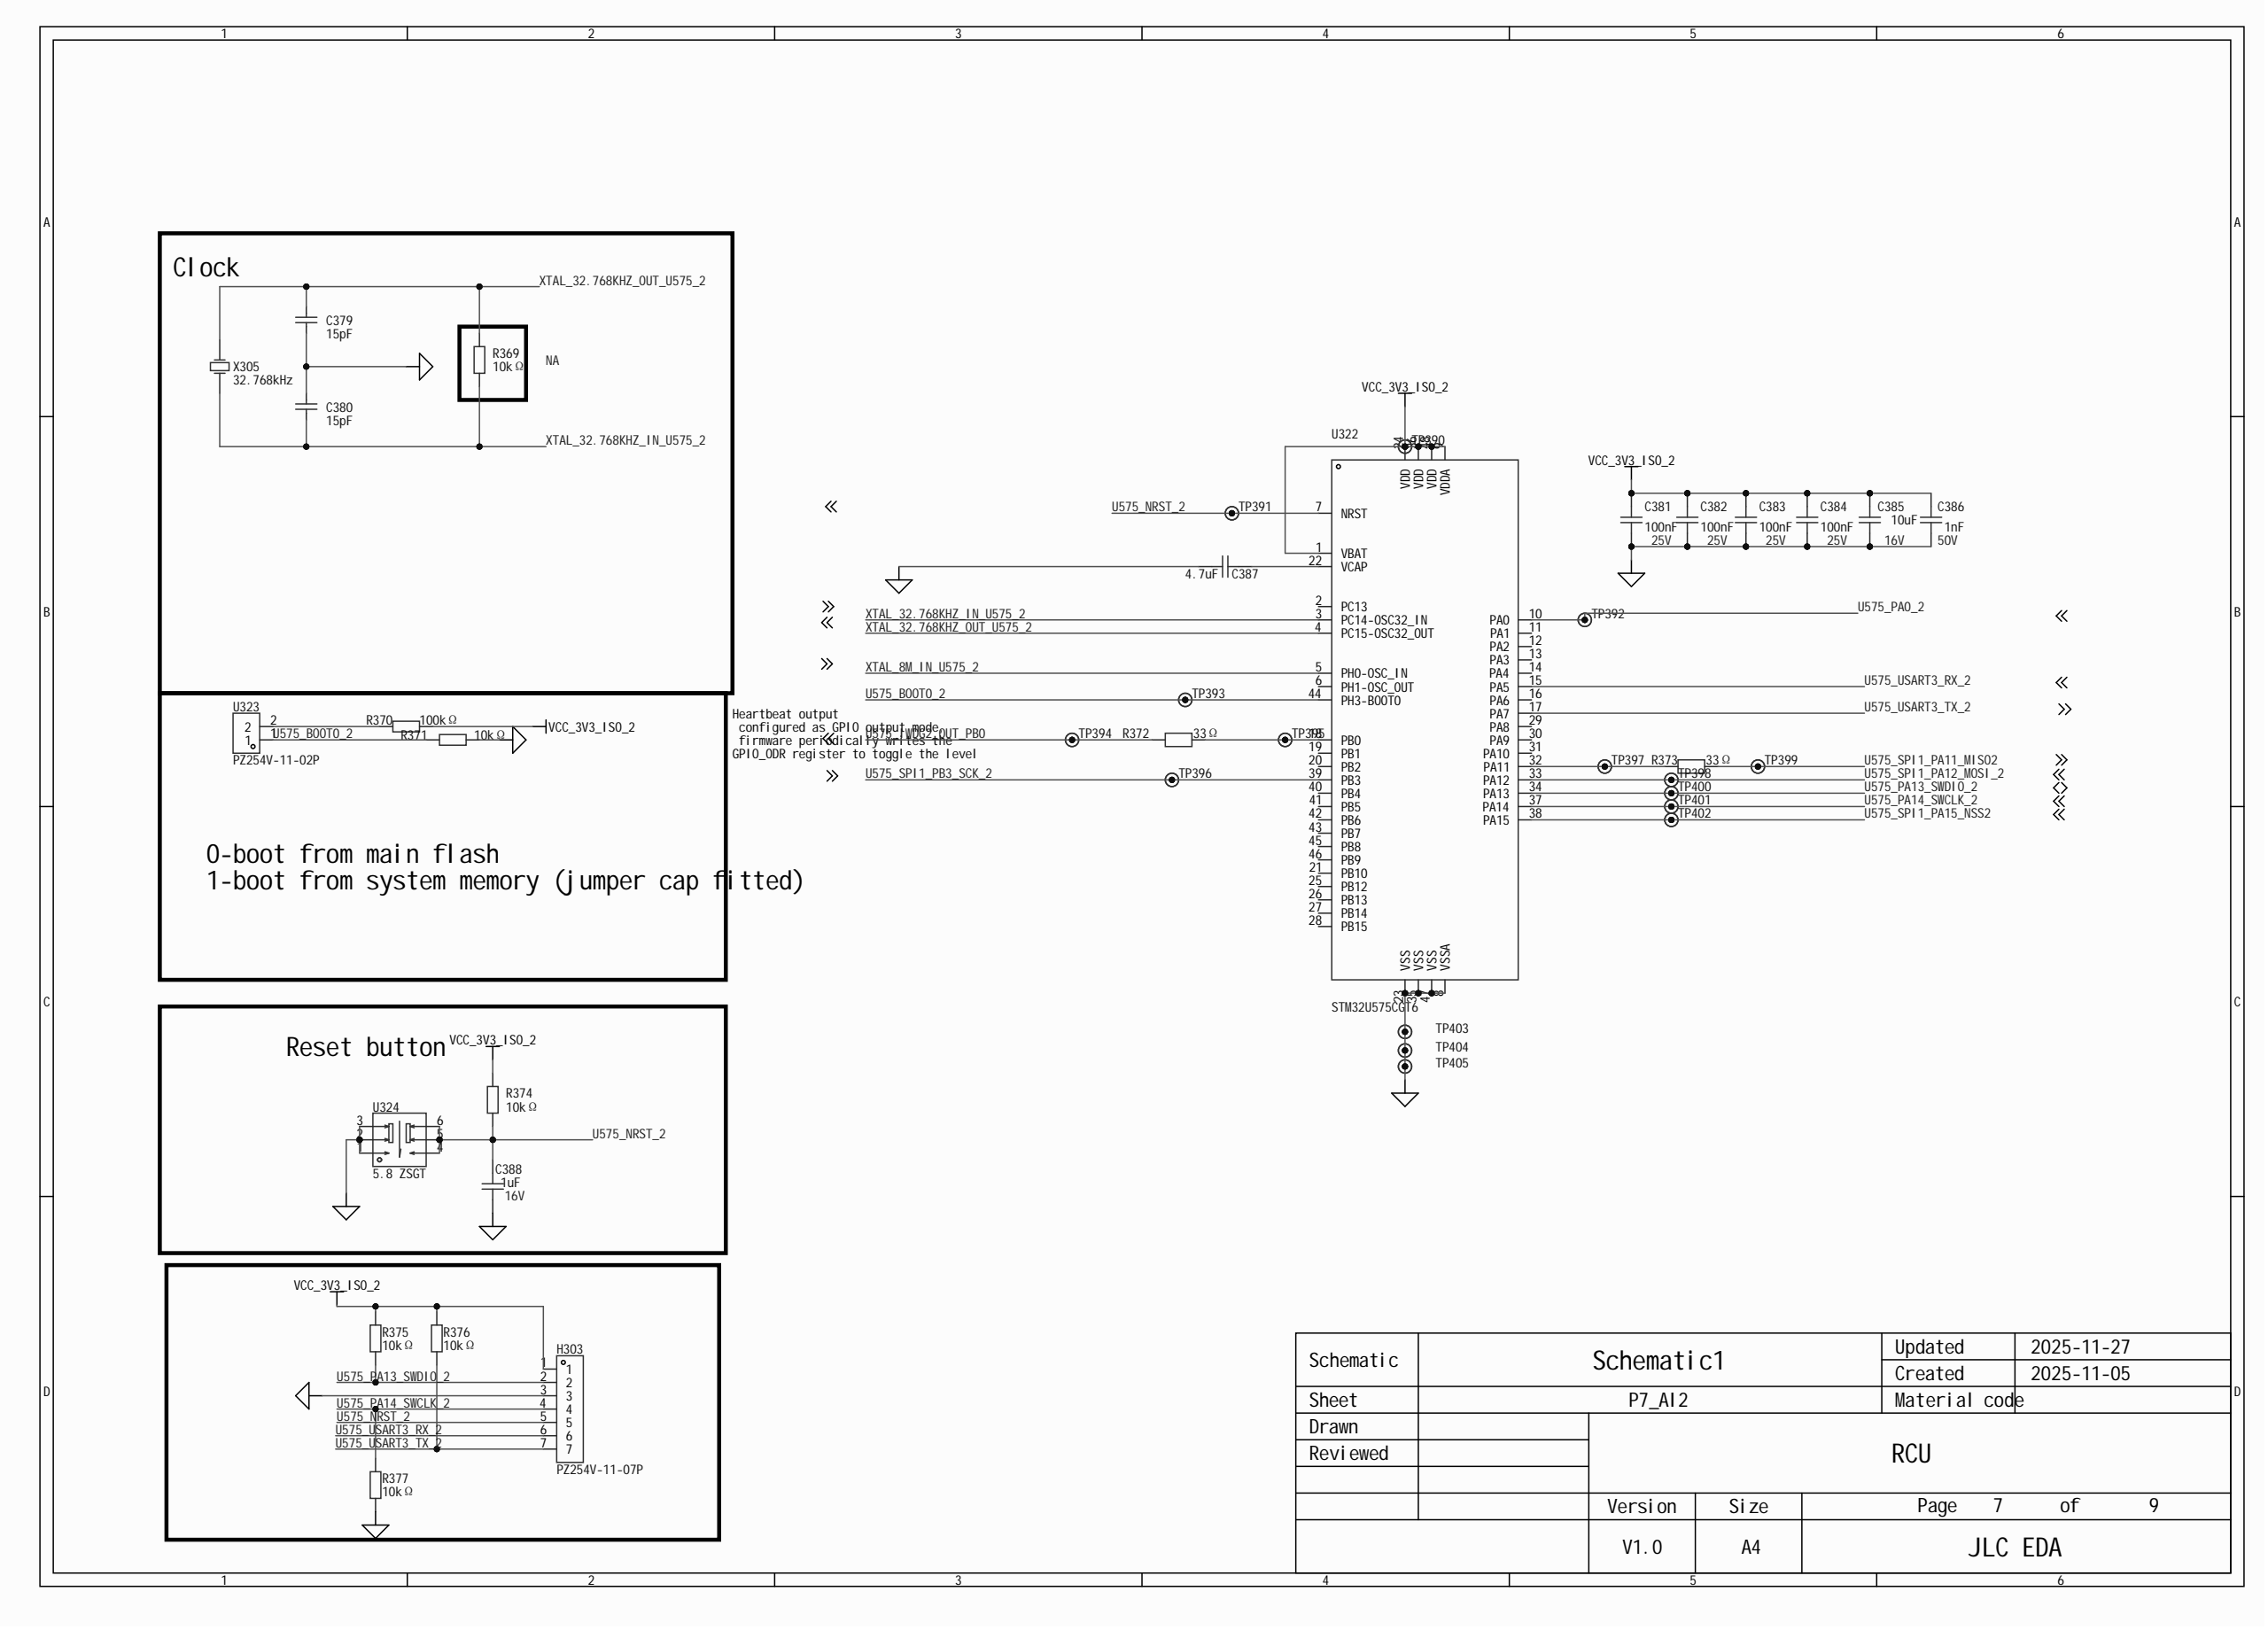Circuit board | Altium Designer | 424 parts | 202 nets | one sheet of the schematic
Parts on this sheet (reference | value | footprint):
C379 | 15pF | C0402
C380 | 15pF | C0402
C381 | 100nF | C0603
C382 | 100nF | C0603
C383 | 100nF | C0603
C384 | 100nF | C0603
C385 | 10uF | C0805
C386 | 1nF | C0603
C387 | 4.7uF | C0603
C388 | 1uF | C0603
H303 | PZ254V-11-07P | HDR-TH_7P-P2.54-V-M
R369 | 10kΩ | R0402
R370 | 100kΩ | R0603
R371 | 10kΩ | R0603
R372 | 33Ω | R0603
R373 | 33Ω | R0603
R374 | 10kΩ | R0402
R375 | 10kΩ | R0603
R376 | 10kΩ | R0603
R377 | 10kΩ | R0603
TP390 | Test-Point-0.5mm
TP391 | Test-Point-0.5mm
TP392 | Test-Point-0.5mm
TP393 | Test-Point-0.5mm
TP394 | Test-Point-0.5mm
TP395 | Test-Point-0.5mm
TP396 | Test-Point-0.5mm
TP397 | Test-Point-0.5mm
TP398 | Test-Point-0.5mm
TP399 | Test-Point-0.5mm
TP400 | Test-Point-0.5mm
TP401 | Test-Point-0.5mm
TP402 | Test-Point-0.5mm
TP403 | Test-Point-0.5mm
TP404 | Test-Point-0.5mm
TP405 | Test-Point-0.5mm
U322 | STM32U575CGT6 | LQFP-48_L7.0-W7.0-P0.50-LS9.0-TL
U323 | PZ254V-11-02P | HDR-TH_2P-P2.54-V-M
U324 | 5.8 ZSGT | SW-TH_5.8ZSGT
X305 | 32.768kHz | OSC-TH_BD3.1-P0.8-D0.3
Nets of these parts (net: part-pin ...):
XTAL_32.768KHZ_OUT_U575_2: C379-2 R369-2 X305-2 U322-4
XTAL_32.768KHZ_IN_U575_2: C380-1 R369-1 X305-1 U322-3
XTAL_8M_IN_U575_2: U322-5
VCC_3V3_ISO_2: C381-1 C382-1 C383-1 C384-1 C385-2 C386-2 H303-1 R370-2 R374-2 R375-2 R376-2 TP390-1 U322-1 U322-9 U322-24 U322-36 U322-48
U575_USART3_TX_2: H303-7 R376-1 U322-17
U575_USART3_RX_2: H303-6 U322-15
U575_SPI1_PB3_SCK_2: TP396-1 U322-39
U575_SPI1_PA15_NSS2: TP402-1 U322-38
U575_SPI1_PA12_MOSI_2: TP398-1 U322-33
U575_SPI1_PA11_MISO2: R373-1 TP399-1
U575_PA14_SWCLK_2: H303-4 R377-1 TP401-1 U322-37
U575_PA13_SWDIO_2: H303-2 R375-1 TP400-1 U322-34
U575_PA0_2: TP392-1 U322-10
U575_NRST_2: C388-2 H303-5 R374-1 TP391-1 U324-4 U324-5 U324-6 U322-7
U575_IWDG2_OUT_PB0: R372-2 TP394-1
U575_BOOT0_2: R371-2 TP393-1 U323-1 U322-44
PGND: C379-1 C380-2 C381-2 C382-2 C383-2 C384-2 C385-1 C386-1 C387-2 C388-1 H303-3 R371-1 R377-2 TP403-1 TP404-1 TP405-1 U324-1 U324-2 U324-3 U322-8 U322-23 U322-35 U322-47
NetR373_2: R373-2 TP397-1 U322-32
NetR372_1: R372-1 TP395-1 U322-18
NetR370_1: R370-1 U323-2
NetC387_1: C387-1 U322-22